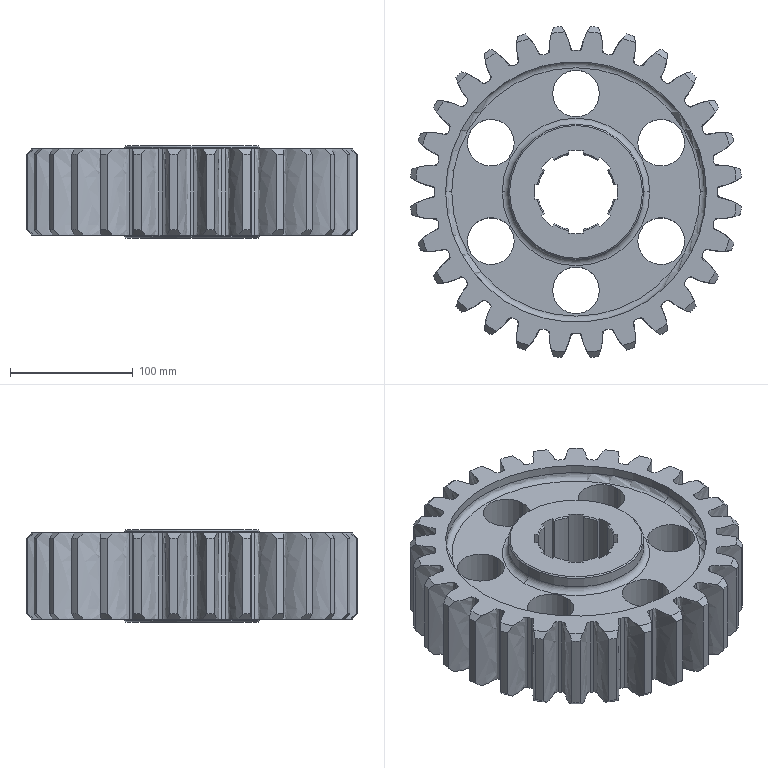Part | SolidWorks | features Chamfer 5, ICE 5, CirPattern 2, Extrusion 1, MirrorPattern 1, RefAxis 1, RevCut 1 | 1 solid | 255 faces | box 268.959 x 268.959 x 75 mm | volume 2318333 mm3 | cylinder 93 | cone 76 | spline 56 | plane 22 | torus 8 | commonest cylinder face diameters 229.5 x28 270 x28 38 x12 68 x9 62 x8 110 x4